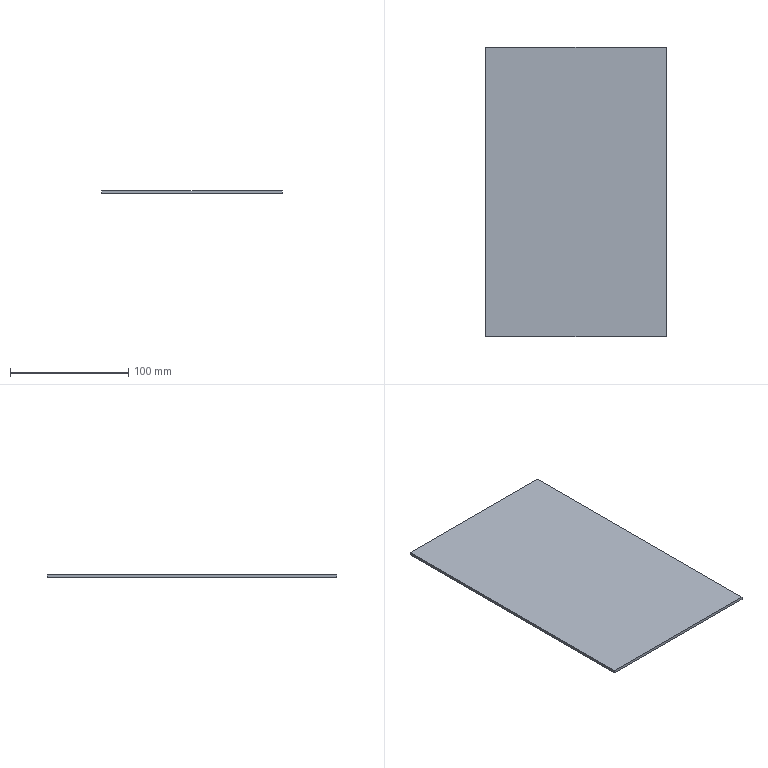Part | SolidWorks | features BaseBody 1 | 1 solid | 11 faces | box 152.5 x 244.9 x 2.34 mm | volume 82614 mm3 | plane 11
STEP:
#1=CARTESIAN_POINT('',(75.85,-123.5,2.2));
#2=VERTEX_POINT('',#1);
#3=CARTESIAN_POINT('',(75.85,121.4,2.2));
#4=VERTEX_POINT('',#3);
#5=CARTESIAN_POINT('',(75.85,0.,2.2));
#6=DIRECTION('',(0.,1.,0.));
#7=VECTOR('',#6,1000.);
#8=LINE('',#5,#7);
#9=EDGE_CURVE('',#2,#4,#8,.T.);
#10=ORIENTED_EDGE('',*,*,#9,.T.);
#11=CARTESIAN_POINT('',(-76.65,121.4,2.2));
#12=VERTEX_POINT('',#11);
#13=CARTESIAN_POINT('',(0.,121.4,2.2));
#14=DIRECTION('',(-1.,0.,0.));
#15=VECTOR('',#14,1000.);
#16=LINE('',#13,#15);
#17=EDGE_CURVE('',#4,#12,#16,.T.);
#18=ORIENTED_EDGE('',*,*,#17,.T.);
#19=CARTESIAN_POINT('',(-76.65,-123.5,2.2));
#20=VERTEX_POINT('',#19);
#21=CARTESIAN_POINT('',(-76.65,0.,2.2));
#22=DIRECTION('',(0.,-1.,0.));
#23=VECTOR('',#22,1000.);
#24=LINE('',#21,#23);
#25=EDGE_CURVE('',#12,#20,#24,.T.);
#26=ORIENTED_EDGE('',*,*,#25,.T.);
#27=CARTESIAN_POINT('',(0.,-123.5,2.2));
#28=DIRECTION('',(1.,0.,0.));
#29=VECTOR('',#28,1000.);
#30=LINE('',#27,#29);
#31=EDGE_CURVE('',#20,#2,#30,.T.);
#32=ORIENTED_EDGE('',*,*,#31,.T.);
#33=EDGE_LOOP('',(#10,#18,#26,#32));
#34=FACE_OUTER_BOUND('',#33,.T.);
#35=CARTESIAN_POINT('',(0.,0.,2.2));
#36=DIRECTION('',(0.,0.,1.));
#37=DIRECTION('',(1.,0.,0.));
#38=AXIS2_PLACEMENT_3D('',#35,#36,#37);
#39=PLANE('',#38);
#40=ADVANCED_FACE('',(#34),#39,.T.);
#41=CARTESIAN_POINT('',(75.85,121.4,-0.14));
#42=VERTEX_POINT('',#41);
#43=CARTESIAN_POINT('',(-76.65,121.4,-0.14));
#44=VERTEX_POINT('',#43);
#45=CARTESIAN_POINT('',(75.85,121.4,-0.14));
#46=DIRECTION('',(-1.,0.,0.));
#47=VECTOR('',#46,1000.);
#48=LINE('',#45,#47);
#49=EDGE_CURVE('',#42,#44,#48,.T.);
#50=ORIENTED_EDGE('',*,*,#49,.T.);
#51=CARTESIAN_POINT('',(-76.65,121.4,0.));
#52=DIRECTION('',(0.,0.,1.));
#53=VECTOR('',#52,1000.);
#54=LINE('',#51,#53);
#55=EDGE_CURVE('',#44,#12,#54,.T.);
#56=ORIENTED_EDGE('',*,*,#55,.T.);
#57=ORIENTED_EDGE('',*,*,#17,.F.);
#58=CARTESIAN_POINT('',(75.85,121.4,0.));
#59=DIRECTION('',(0.,0.,-1.));
#60=VECTOR('',#59,1000.);
#61=LINE('',#58,#60);
#62=EDGE_CURVE('',#4,#42,#61,.T.);
#63=ORIENTED_EDGE('',*,*,#62,.T.);
#64=EDGE_LOOP('',(#50,#56,#57,#63));
#65=FACE_OUTER_BOUND('',#64,.T.);
#66=CARTESIAN_POINT('',(75.85,121.4,0.));
#67=DIRECTION('',(0.,1.,0.));
#68=DIRECTION('',(0.,0.,1.));
#69=AXIS2_PLACEMENT_3D('',#66,#67,#68);
#70=PLANE('',#69);
#71=ADVANCED_FACE('',(#65),#70,.T.);
#72=CARTESIAN_POINT('',(75.85,-123.5,-0.14));
#73=VERTEX_POINT('',#72);
#74=CARTESIAN_POINT('',(75.85,-123.5,-0.14));
#75=DIRECTION('',(0.,1.,0.));
#76=VECTOR('',#75,1000.);
#77=LINE('',#74,#76);
#78=EDGE_CURVE('',#73,#42,#77,.T.);
#79=ORIENTED_EDGE('',*,*,#78,.T.);
#80=ORIENTED_EDGE('',*,*,#62,.F.);
#81=ORIENTED_EDGE('',*,*,#9,.F.);
#82=CARTESIAN_POINT('',(75.85,-123.5,0.));
#83=DIRECTION('',(0.,0.,-1.));
#84=VECTOR('',#83,1000.);
#85=LINE('',#82,#84);
#86=EDGE_CURVE('',#2,#73,#85,.T.);
#87=ORIENTED_EDGE('',*,*,#86,.T.);
#88=EDGE_LOOP('',(#79,#80,#81,#87));
#89=FACE_OUTER_BOUND('',#88,.T.);
#90=CARTESIAN_POINT('',(75.85,-123.5,0.));
#91=DIRECTION('',(1.,0.,0.));
#92=DIRECTION('',(0.,0.,-1.));
#93=AXIS2_PLACEMENT_3D('',#90,#91,#92);
#94=PLANE('',#93);
#95=ADVANCED_FACE('',(#89),#94,.T.);
#96=CARTESIAN_POINT('',(-76.65,-123.5,-0.14));
#97=VERTEX_POINT('',#96);
#98=CARTESIAN_POINT('',(-76.65,-123.5,-0.14));
#99=DIRECTION('',(1.,0.,0.));
#100=VECTOR('',#99,1000.);
#101=LINE('',#98,#100);
#102=EDGE_CURVE('',#97,#73,#101,.T.);
#103=ORIENTED_EDGE('',*,*,#102,.T.);
#104=ORIENTED_EDGE('',*,*,#86,.F.);
#105=ORIENTED_EDGE('',*,*,#31,.F.);
#106=CARTESIAN_POINT('',(-76.65,-123.5,0.));
#107=DIRECTION('',(0.,0.,-1.));
#108=VECTOR('',#107,1000.);
#109=LINE('',#106,#108);
#110=EDGE_CURVE('',#20,#97,#109,.T.);
#111=ORIENTED_EDGE('',*,*,#110,.T.);
#112=EDGE_LOOP('',(#103,#104,#105,#111));
#113=FACE_OUTER_BOUND('',#112,.T.);
#114=CARTESIAN_POINT('',(-76.65,-123.5,0.));
#115=DIRECTION('',(0.,-1.,0.));
#116=DIRECTION('',(0.,0.,-1.));
#117=AXIS2_PLACEMENT_3D('',#114,#115,#116);
#118=PLANE('',#117);
#119=ADVANCED_FACE('',(#113),#118,.T.);
#120=CARTESIAN_POINT('',(-76.65,121.4,-0.14));
#121=DIRECTION('',(0.,-1.,0.));
#122=VECTOR('',#121,1000.);
#123=LINE('',#120,#122);
#124=EDGE_CURVE('',#44,#97,#123,.T.);
#125=ORIENTED_EDGE('',*,*,#124,.T.);
#126=ORIENTED_EDGE('',*,*,#110,.F.);
#127=ORIENTED_EDGE('',*,*,#25,.F.);
#128=ORIENTED_EDGE('',*,*,#55,.F.);
#129=EDGE_LOOP('',(#125,#126,#127,#128));
#130=FACE_OUTER_BOUND('',#129,.T.);
#131=CARTESIAN_POINT('',(-76.65,121.4,0.));
#132=DIRECTION('',(-1.,0.,0.));
#133=DIRECTION('',(0.,0.,1.));
#134=AXIS2_PLACEMENT_3D('',#131,#132,#133);
#135=PLANE('',#134);
#136=ADVANCED_FACE('',(#130),#135,.T.);
#137=CARTESIAN_POINT('',(-71.8,-118.8,-0.14));
#138=VERTEX_POINT('',#137);
#139=CARTESIAN_POINT('',(72.6,-118.8,-0.14));
#140=VERTEX_POINT('',#139);
#141=CARTESIAN_POINT('',(0.,-118.8,-0.14));
#142=DIRECTION('',(1.,0.,0.));
#143=VECTOR('',#142,1000.);
#144=LINE('',#141,#143);
#145=EDGE_CURVE('',#138,#140,#144,.T.);
#146=ORIENTED_EDGE('',*,*,#145,.T.);
#147=CARTESIAN_POINT('',(72.6,117.6,-0.14));
#148=VERTEX_POINT('',#147);
#149=CARTESIAN_POINT('',(72.6,0.,-0.14));
#150=DIRECTION('',(0.,1.,0.));
#151=VECTOR('',#150,1000.);
#152=LINE('',#149,#151);
#153=EDGE_CURVE('',#140,#148,#152,.T.);
#154=ORIENTED_EDGE('',*,*,#153,.T.);
#155=CARTESIAN_POINT('',(-71.8,117.6,-0.14));
#156=VERTEX_POINT('',#155);
#157=CARTESIAN_POINT('',(0.,117.6,-0.14));
#158=DIRECTION('',(-1.,0.,0.));
#159=VECTOR('',#158,1000.);
#160=LINE('',#157,#159);
#161=EDGE_CURVE('',#148,#156,#160,.T.);
#162=ORIENTED_EDGE('',*,*,#161,.T.);
#163=CARTESIAN_POINT('',(-71.8,0.,-0.14));
#164=DIRECTION('',(0.,-1.,0.));
#165=VECTOR('',#164,1000.);
#166=LINE('',#163,#165);
#167=EDGE_CURVE('',#156,#138,#166,.T.);
#168=ORIENTED_EDGE('',*,*,#167,.T.);
#169=EDGE_LOOP('',(#146,#154,#162,#168));
#170=FACE_BOUND('',#169,.T.);
#171=ORIENTED_EDGE('',*,*,#49,.F.);
#172=ORIENTED_EDGE('',*,*,#78,.F.);
#173=ORIENTED_EDGE('',*,*,#102,.F.);
#174=ORIENTED_EDGE('',*,*,#124,.F.);
#175=EDGE_LOOP('',(#171,#172,#173,#174));
#176=FACE_OUTER_BOUND('',#175,.T.);
#177=CARTESIAN_POINT('',(0.,0.,-0.14));
#178=DIRECTION('',(0.,0.,-1.));
#179=DIRECTION('',(-1.,0.,0.));
#180=AXIS2_PLACEMENT_3D('',#177,#178,#179);
#181=PLANE('',#180);
#182=ADVANCED_FACE('',(#170,#176),#181,.T.);
#183=CARTESIAN_POINT('',(72.6,-118.8,0.));
#184=VERTEX_POINT('',#183);
#185=CARTESIAN_POINT('',(72.6,-118.8,0.));
#186=DIRECTION('',(0.,0.,1.));
#187=VECTOR('',#186,1000.);
#188=LINE('',#185,#187);
#189=EDGE_CURVE('',#140,#184,#188,.T.);
#190=ORIENTED_EDGE('',*,*,#189,.T.);
#191=CARTESIAN_POINT('',(72.6,117.6,0.));
#192=VERTEX_POINT('',#191);
#193=CARTESIAN_POINT('',(72.6,-118.8,0.));
#194=DIRECTION('',(0.,1.,0.));
#195=VECTOR('',#194,1000.);
#196=LINE('',#193,#195);
#197=EDGE_CURVE('',#184,#192,#196,.T.);
#198=ORIENTED_EDGE('',*,*,#197,.T.);
#199=CARTESIAN_POINT('',(72.6,117.6,0.));
#200=DIRECTION('',(0.,0.,-1.));
#201=VECTOR('',#200,1000.);
#202=LINE('',#199,#201);
#203=EDGE_CURVE('',#192,#148,#202,.T.);
#204=ORIENTED_EDGE('',*,*,#203,.T.);
#205=ORIENTED_EDGE('',*,*,#153,.F.);
#206=EDGE_LOOP('',(#190,#198,#204,#205));
#207=FACE_OUTER_BOUND('',#206,.T.);
#208=CARTESIAN_POINT('',(72.6,-118.8,0.));
#209=DIRECTION('',(-1.,0.,0.));
#210=DIRECTION('',(0.,0.,1.));
#211=AXIS2_PLACEMENT_3D('',#208,#209,#210);
#212=PLANE('',#211);
#213=ADVANCED_FACE('',(#207),#212,.T.);
#214=CARTESIAN_POINT('',(-71.8,-118.8,0.));
#215=VERTEX_POINT('',#214);
#216=CARTESIAN_POINT('',(-71.8,-118.8,0.));
#217=DIRECTION('',(0.,0.,1.));
#218=VECTOR('',#217,1000.);
#219=LINE('',#216,#218);
#220=EDGE_CURVE('',#138,#215,#219,.T.);
#221=ORIENTED_EDGE('',*,*,#220,.T.);
#222=CARTESIAN_POINT('',(-71.8,-118.8,0.));
#223=DIRECTION('',(1.,0.,0.));
#224=VECTOR('',#223,1000.);
#225=LINE('',#222,#224);
#226=EDGE_CURVE('',#215,#184,#225,.T.);
#227=ORIENTED_EDGE('',*,*,#226,.T.);
#228=ORIENTED_EDGE('',*,*,#189,.F.);
#229=ORIENTED_EDGE('',*,*,#145,.F.);
#230=EDGE_LOOP('',(#221,#227,#228,#229));
#231=FACE_OUTER_BOUND('',#230,.T.);
#232=CARTESIAN_POINT('',(-71.8,-118.8,0.));
#233=DIRECTION('',(0.,1.,0.));
#234=DIRECTION('',(0.,0.,1.));
#235=AXIS2_PLACEMENT_3D('',#232,#233,#234);
#236=PLANE('',#235);
#237=ADVANCED_FACE('',(#231),#236,.T.);
#238=CARTESIAN_POINT('',(-71.8,117.6,0.));
#239=VERTEX_POINT('',#238);
#240=CARTESIAN_POINT('',(-71.8,117.6,0.));
#241=DIRECTION('',(0.,0.,1.));
#242=VECTOR('',#241,1000.);
#243=LINE('',#240,#242);
#244=EDGE_CURVE('',#156,#239,#243,.T.);
#245=ORIENTED_EDGE('',*,*,#244,.T.);
#246=CARTESIAN_POINT('',(-71.8,117.6,0.));
#247=DIRECTION('',(0.,-1.,0.));
#248=VECTOR('',#247,1000.);
#249=LINE('',#246,#248);
#250=EDGE_CURVE('',#239,#215,#249,.T.);
#251=ORIENTED_EDGE('',*,*,#250,.T.);
#252=ORIENTED_EDGE('',*,*,#220,.F.);
#253=ORIENTED_EDGE('',*,*,#167,.F.);
#254=EDGE_LOOP('',(#245,#251,#252,#253));
#255=FACE_OUTER_BOUND('',#254,.T.);
#256=CARTESIAN_POINT('',(-71.8,117.6,0.));
#257=DIRECTION('',(1.,0.,0.));
#258=DIRECTION('',(0.,0.,-1.));
#259=AXIS2_PLACEMENT_3D('',#256,#257,#258);
#260=PLANE('',#259);
#261=ADVANCED_FACE('',(#255),#260,.T.);
#262=ORIENTED_EDGE('',*,*,#203,.F.);
#263=CARTESIAN_POINT('',(72.6,117.6,0.));
#264=DIRECTION('',(-1.,0.,0.));
#265=VECTOR('',#264,1000.);
#266=LINE('',#263,#265);
#267=EDGE_CURVE('',#192,#239,#266,.T.);
#268=ORIENTED_EDGE('',*,*,#267,.T.);
#269=ORIENTED_EDGE('',*,*,#244,.F.);
#270=ORIENTED_EDGE('',*,*,#161,.F.);
#271=EDGE_LOOP('',(#262,#268,#269,#270));
#272=FACE_OUTER_BOUND('',#271,.T.);
#273=CARTESIAN_POINT('',(72.6,117.6,0.));
#274=DIRECTION('',(0.,-1.,0.));
#275=DIRECTION('',(0.,0.,-1.));
#276=AXIS2_PLACEMENT_3D('',#273,#274,#275);
#277=PLANE('',#276);
#278=ADVANCED_FACE('',(#272),#277,.T.);
#279=ORIENTED_EDGE('',*,*,#267,.F.);
#280=ORIENTED_EDGE('',*,*,#197,.F.);
#281=ORIENTED_EDGE('',*,*,#226,.F.);
#282=ORIENTED_EDGE('',*,*,#250,.F.);
#283=EDGE_LOOP('',(#279,#280,#281,#282));
#284=FACE_OUTER_BOUND('',#283,.T.);
#285=CARTESIAN_POINT('',(0.,0.,0.));
#286=DIRECTION('',(0.,0.,1.));
#287=DIRECTION('',(1.,0.,0.));
#288=AXIS2_PLACEMENT_3D('',#285,#286,#287);
#289=PLANE('',#288);
#290=ADVANCED_FACE('',(#284),#289,.F.);
#291=CLOSED_SHELL('',(#40,#71,#95,#119,#136,#182,#213,#237,#261,#278,#290));
#292=MANIFOLD_SOLID_BREP('',#291);
#293=CARTESIAN_POINT('',(0.,0.,0.));
#294=DIRECTION('',(0.,0.,1.));
#295=DIRECTION('',(1.,0.,0.));
#296=AXIS2_PLACEMENT_3D('',#293,#294,#295);
#297=(LENGTH_UNIT()NAMED_UNIT(*)SI_UNIT(.MILLI.,.METRE.));
#298=UNCERTAINTY_MEASURE_WITH_UNIT(LENGTH_MEASURE(0.00001),#297,'','');
#299=(NAMED_UNIT(*)PLANE_ANGLE_UNIT()SI_UNIT($,.RADIAN.));
#300=(NAMED_UNIT(*)SI_UNIT($,.STERADIAN.)SOLID_ANGLE_UNIT());
#301=(GEOMETRIC_REPRESENTATION_CONTEXT(3)GLOBAL_UNCERTAINTY_ASSIGNED_CONTEXT((#298))GLOBAL_UNIT_ASSIGNED_CONTEXT((#297,#299,#300))REPRESENTATION_CONTEXT('',''));
#302=ADVANCED_BREP_SHAPE_REPRESENTATION('',(#292,#296),#301);